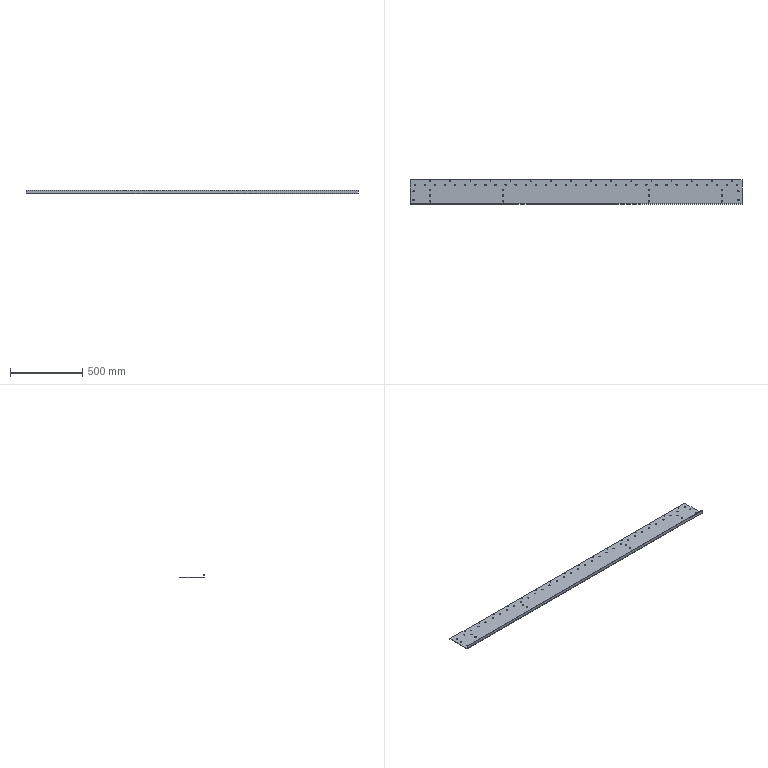Part | STEP file | cc-roller-32 | 1 solid | 75 faces | box 2303 x 170 x 25 mm | volume 1090692 mm3 | spline 65 | plane 8 | cylinder 2 | commonest cylinder face diameters 5 x1 10 x1